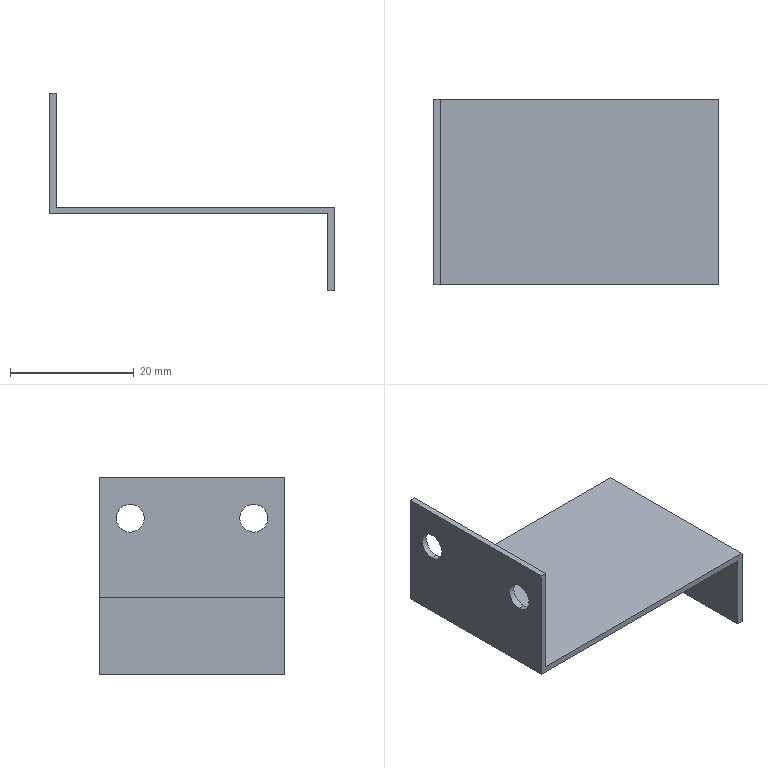Part | STEP file | 0244_221_Dog | 1 solid | 14 faces | box 46 x 30 x 32 mm | volume 2278 mm3 | plane 10 | cylinder 4 | commonest cylinder face diameters 4.5 x4
STEP:
#1=CARTESIAN_POINT('',(0.,0.,0.));
#2=DIRECTION('',(0.,0.,1.));
#3=DIRECTION('',(1.,0.,0.));
#4=AXIS2_PLACEMENT_3D('',#1,#2,#3);
#5=CARTESIAN_POINT('',(0.,10.,10.6));
#6=VERTEX_POINT('',#5);
#7=CARTESIAN_POINT('',(1.,10.,10.6));
#8=VERTEX_POINT('',#7);
#9=CARTESIAN_POINT('',(1.,10.,10.6));
#10=DIRECTION('',(1.,0.,0.));
#11=VECTOR('',#10,1.);
#12=LINE('',#9,#11);
#13=CARTESIAN_POINT('',(1.,10.,12.85));
#14=DIRECTION('',(1.,0.,0.));
#15=DIRECTION('',(0.,0.,-1.));
#16=AXIS2_PLACEMENT_3D('',#13,#14,#15);
#17=CYLINDRICAL_SURFACE('',#16,2.25);
#18=CARTESIAN_POINT('',(6.283,0.));
#19=DIRECTION('',(0.,1.));
#20=VECTOR('',#19,1.);
#21=LINE('',#18,#20);
#22=(GEOMETRIC_REPRESENTATION_CONTEXT(2)PARAMETRIC_REPRESENTATION_CONTEXT()REPRESENTATION_CONTEXT('',''));
#23=DEFINITIONAL_REPRESENTATION('',(#21),#22);
#24=PCURVE('',#17,#23);
#25=CARTESIAN_POINT('',(1.,10.,12.85));
#26=DIRECTION('',(1.,0.,0.));
#27=DIRECTION('',(0.,0.,-1.));
#28=AXIS2_PLACEMENT_3D('',#25,#26,#27);
#29=CYLINDRICAL_SURFACE('',#28,2.25);
#30=CARTESIAN_POINT('',(0.,0.));
#31=DIRECTION('',(0.,1.));
#32=VECTOR('',#31,1.);
#33=LINE('',#30,#32);
#34=(GEOMETRIC_REPRESENTATION_CONTEXT(2)PARAMETRIC_REPRESENTATION_CONTEXT()REPRESENTATION_CONTEXT('',''));
#35=DEFINITIONAL_REPRESENTATION('',(#33),#34);
#36=PCURVE('',#29,#35);
#37=SURFACE_CURVE('',#12,(#24,#36),.PCURVE_S1.);
#38=EDGE_CURVE('',#6,#8,#37,.T.);
#39=ORIENTED_EDGE('',*,*,#38,.T.);
#40=CARTESIAN_POINT('',(1.,10.,15.1));
#41=VERTEX_POINT('',#40);
#42=CARTESIAN_POINT('',(1.,10.,12.85));
#43=DIRECTION('',(1.,0.,0.));
#44=DIRECTION('',(0.,0.,-1.));
#45=AXIS2_PLACEMENT_3D('',#42,#43,#44);
#46=CIRCLE('',#45,2.25);
#47=CARTESIAN_POINT('',(0.,0.));
#48=DIRECTION('',(1.,0.));
#49=VECTOR('',#48,1.);
#50=LINE('',#47,#49);
#51=(GEOMETRIC_REPRESENTATION_CONTEXT(2)PARAMETRIC_REPRESENTATION_CONTEXT()REPRESENTATION_CONTEXT('',''));
#52=DEFINITIONAL_REPRESENTATION('',(#50),#51);
#53=PCURVE('',#17,#52);
#54=CARTESIAN_POINT('',(1.,15.,1.));
#55=DIRECTION('',(-1.,0.,0.));
#56=DIRECTION('',(0.,0.,1.));
#57=AXIS2_PLACEMENT_3D('',#54,#55,#56);
#58=PLANE('',#57);
#59=CARTESIAN_POINT('',(9.6,-5.));
#60=CARTESIAN_POINT('',(9.6,-1.103));
#61=CARTESIAN_POINT('',(12.975,-3.051));
#62=CARTESIAN_POINT('',(16.35,-5.));
#63=CARTESIAN_POINT('',(12.975,-6.949));
#64=CARTESIAN_POINT('',(9.6,-8.897));
#65=CARTESIAN_POINT('',(9.6,-5.));
#66=(BOUNDED_CURVE()B_SPLINE_CURVE(2,(#59,#60,#61,#62,#63,#64,#65),.UNSPECIFIED.,.T.,.F.)B_SPLINE_CURVE_WITH_KNOTS((1,2,2,2,2,1),(-2.094,0.,2.094,4.189,6.283,8.378),.UNSPECIFIED.)CURVE()GEOMETRIC_REPRESENTATION_ITEM()RATIONAL_B_SPLINE_CURVE((1.,0.5,1.,0.5,1.,0.5,1.))REPRESENTATION_ITEM(''));
#67=(GEOMETRIC_REPRESENTATION_CONTEXT(2)PARAMETRIC_REPRESENTATION_CONTEXT()REPRESENTATION_CONTEXT('',''));
#68=DEFINITIONAL_REPRESENTATION('',(#66),#67);
#69=PCURVE('',#58,#68);
#70=SURFACE_CURVE('',#46,(#53,#69),.PCURVE_S1.);
#71=EDGE_CURVE('',#41,#8,#70,.T.);
#72=ORIENTED_EDGE('',*,*,#71,.F.);
#73=CARTESIAN_POINT('',(0.,10.,15.1));
#74=VERTEX_POINT('',#73);
#75=CARTESIAN_POINT('',(1.,10.,15.1));
#76=DIRECTION('',(1.,0.,0.));
#77=VECTOR('',#76,1.);
#78=LINE('',#75,#77);
#79=CARTESIAN_POINT('',(3.142,0.));
#80=DIRECTION('',(0.,1.));
#81=VECTOR('',#80,1.);
#82=LINE('',#79,#81);
#83=(GEOMETRIC_REPRESENTATION_CONTEXT(2)PARAMETRIC_REPRESENTATION_CONTEXT()REPRESENTATION_CONTEXT('',''));
#84=DEFINITIONAL_REPRESENTATION('',(#82),#83);
#85=PCURVE('',#17,#84);
#86=CARTESIAN_POINT('',(3.142,0.));
#87=DIRECTION('',(0.,1.));
#88=VECTOR('',#87,1.);
#89=LINE('',#86,#88);
#90=(GEOMETRIC_REPRESENTATION_CONTEXT(2)PARAMETRIC_REPRESENTATION_CONTEXT()REPRESENTATION_CONTEXT('',''));
#91=DEFINITIONAL_REPRESENTATION('',(#89),#90);
#92=PCURVE('',#29,#91);
#93=SURFACE_CURVE('',#78,(#85,#92),.PCURVE_S1.);
#94=EDGE_CURVE('',#74,#41,#93,.T.);
#95=ORIENTED_EDGE('',*,*,#94,.F.);
#96=CARTESIAN_POINT('',(0.,10.,12.85));
#97=DIRECTION('',(1.,0.,0.));
#98=DIRECTION('',(0.,0.,-1.));
#99=AXIS2_PLACEMENT_3D('',#96,#97,#98);
#100=CIRCLE('',#99,2.25);
#101=CARTESIAN_POINT('',(0.,-1.));
#102=DIRECTION('',(1.,0.));
#103=VECTOR('',#102,1.);
#104=LINE('',#101,#103);
#105=(GEOMETRIC_REPRESENTATION_CONTEXT(2)PARAMETRIC_REPRESENTATION_CONTEXT()REPRESENTATION_CONTEXT('',''));
#106=DEFINITIONAL_REPRESENTATION('',(#104),#105);
#107=PCURVE('',#17,#106);
#108=CARTESIAN_POINT('',(0.,15.,0.));
#109=DIRECTION('',(1.,0.,0.));
#110=DIRECTION('',(0.,0.,-1.));
#111=AXIS2_PLACEMENT_3D('',#108,#109,#110);
#112=PLANE('',#111);
#113=CARTESIAN_POINT('',(-12.85,-5.));
#114=DIRECTION('',(1.,0.));
#115=AXIS2_PLACEMENT_2D('',#113,#114);
#116=CIRCLE('',#115,2.25);
#117=(GEOMETRIC_REPRESENTATION_CONTEXT(2)PARAMETRIC_REPRESENTATION_CONTEXT()REPRESENTATION_CONTEXT('',''));
#118=DEFINITIONAL_REPRESENTATION('',(#116),#117);
#119=PCURVE('',#112,#118);
#120=SURFACE_CURVE('',#100,(#107,#119),.PCURVE_S1.);
#121=EDGE_CURVE('',#74,#6,#120,.T.);
#122=ORIENTED_EDGE('',*,*,#121,.T.);
#123=EDGE_LOOP('',(#39,#72,#95,#122));
#124=FACE_BOUND('',#123,.F.);
#125=ADVANCED_FACE('',(#124),#17,.F.);
#126=CARTESIAN_POINT('',(0.,-10.,10.6));
#127=VERTEX_POINT('',#126);
#128=CARTESIAN_POINT('',(1.,-10.,10.6));
#129=VERTEX_POINT('',#128);
#130=CARTESIAN_POINT('',(1.,-10.,10.6));
#131=DIRECTION('',(1.,0.,0.));
#132=VECTOR('',#131,1.);
#133=LINE('',#130,#132);
#134=CARTESIAN_POINT('',(1.,-10.,12.85));
#135=DIRECTION('',(1.,0.,0.));
#136=DIRECTION('',(0.,0.,-1.));
#137=AXIS2_PLACEMENT_3D('',#134,#135,#136);
#138=CYLINDRICAL_SURFACE('',#137,2.25);
#139=CARTESIAN_POINT('',(6.283,0.));
#140=DIRECTION('',(0.,1.));
#141=VECTOR('',#140,1.);
#142=LINE('',#139,#141);
#143=(GEOMETRIC_REPRESENTATION_CONTEXT(2)PARAMETRIC_REPRESENTATION_CONTEXT()REPRESENTATION_CONTEXT('',''));
#144=DEFINITIONAL_REPRESENTATION('',(#142),#143);
#145=PCURVE('',#138,#144);
#146=CARTESIAN_POINT('',(1.,-10.,12.85));
#147=DIRECTION('',(1.,0.,0.));
#148=DIRECTION('',(0.,0.,-1.));
#149=AXIS2_PLACEMENT_3D('',#146,#147,#148);
#150=CYLINDRICAL_SURFACE('',#149,2.25);
#151=CARTESIAN_POINT('',(0.,0.));
#152=DIRECTION('',(0.,1.));
#153=VECTOR('',#152,1.);
#154=LINE('',#151,#153);
#155=(GEOMETRIC_REPRESENTATION_CONTEXT(2)PARAMETRIC_REPRESENTATION_CONTEXT()REPRESENTATION_CONTEXT('',''));
#156=DEFINITIONAL_REPRESENTATION('',(#154),#155);
#157=PCURVE('',#150,#156);
#158=SURFACE_CURVE('',#133,(#145,#157),.PCURVE_S1.);
#159=EDGE_CURVE('',#127,#129,#158,.T.);
#160=ORIENTED_EDGE('',*,*,#159,.T.);
#161=CARTESIAN_POINT('',(1.,-10.,15.1));
#162=VERTEX_POINT('',#161);
#163=CARTESIAN_POINT('',(1.,-10.,12.85));
#164=DIRECTION('',(1.,0.,0.));
#165=DIRECTION('',(0.,0.,-1.));
#166=AXIS2_PLACEMENT_3D('',#163,#164,#165);
#167=CIRCLE('',#166,2.25);
#168=CARTESIAN_POINT('',(0.,0.));
#169=DIRECTION('',(1.,0.));
#170=VECTOR('',#169,1.);
#171=LINE('',#168,#170);
#172=(GEOMETRIC_REPRESENTATION_CONTEXT(2)PARAMETRIC_REPRESENTATION_CONTEXT()REPRESENTATION_CONTEXT('',''));
#173=DEFINITIONAL_REPRESENTATION('',(#171),#172);
#174=PCURVE('',#138,#173);
#175=CARTESIAN_POINT('',(9.6,-25.));
#176=CARTESIAN_POINT('',(9.6,-21.103));
#177=CARTESIAN_POINT('',(12.975,-23.051));
#178=CARTESIAN_POINT('',(16.35,-25.));
#179=CARTESIAN_POINT('',(12.975,-26.949));
#180=CARTESIAN_POINT('',(9.6,-28.897));
#181=CARTESIAN_POINT('',(9.6,-25.));
#182=(BOUNDED_CURVE()B_SPLINE_CURVE(2,(#175,#176,#177,#178,#179,#180,#181),.UNSPECIFIED.,.T.,.F.)B_SPLINE_CURVE_WITH_KNOTS((1,2,2,2,2,1),(-2.094,0.,2.094,4.189,6.283,8.378),.UNSPECIFIED.)CURVE()GEOMETRIC_REPRESENTATION_ITEM()RATIONAL_B_SPLINE_CURVE((1.,0.5,1.,0.5,1.,0.5,1.))REPRESENTATION_ITEM(''));
#183=(GEOMETRIC_REPRESENTATION_CONTEXT(2)PARAMETRIC_REPRESENTATION_CONTEXT()REPRESENTATION_CONTEXT('',''));
#184=DEFINITIONAL_REPRESENTATION('',(#182),#183);
#185=PCURVE('',#58,#184);
#186=SURFACE_CURVE('',#167,(#174,#185),.PCURVE_S1.);
#187=EDGE_CURVE('',#162,#129,#186,.T.);
#188=ORIENTED_EDGE('',*,*,#187,.F.);
#189=CARTESIAN_POINT('',(0.,-10.,15.1));
#190=VERTEX_POINT('',#189);
#191=CARTESIAN_POINT('',(1.,-10.,15.1));
#192=DIRECTION('',(1.,0.,0.));
#193=VECTOR('',#192,1.);
#194=LINE('',#191,#193);
#195=CARTESIAN_POINT('',(3.142,0.));
#196=DIRECTION('',(0.,1.));
#197=VECTOR('',#196,1.);
#198=LINE('',#195,#197);
#199=(GEOMETRIC_REPRESENTATION_CONTEXT(2)PARAMETRIC_REPRESENTATION_CONTEXT()REPRESENTATION_CONTEXT('',''));
#200=DEFINITIONAL_REPRESENTATION('',(#198),#199);
#201=PCURVE('',#138,#200);
#202=CARTESIAN_POINT('',(3.142,0.));
#203=DIRECTION('',(0.,1.));
#204=VECTOR('',#203,1.);
#205=LINE('',#202,#204);
#206=(GEOMETRIC_REPRESENTATION_CONTEXT(2)PARAMETRIC_REPRESENTATION_CONTEXT()REPRESENTATION_CONTEXT('',''));
#207=DEFINITIONAL_REPRESENTATION('',(#205),#206);
#208=PCURVE('',#150,#207);
#209=SURFACE_CURVE('',#194,(#201,#208),.PCURVE_S1.);
#210=EDGE_CURVE('',#190,#162,#209,.T.);
#211=ORIENTED_EDGE('',*,*,#210,.F.);
#212=CARTESIAN_POINT('',(0.,-10.,12.85));
#213=DIRECTION('',(1.,0.,0.));
#214=DIRECTION('',(0.,0.,-1.));
#215=AXIS2_PLACEMENT_3D('',#212,#213,#214);
#216=CIRCLE('',#215,2.25);
#217=CARTESIAN_POINT('',(0.,-1.));
#218=DIRECTION('',(1.,0.));
#219=VECTOR('',#218,1.);
#220=LINE('',#217,#219);
#221=(GEOMETRIC_REPRESENTATION_CONTEXT(2)PARAMETRIC_REPRESENTATION_CONTEXT()REPRESENTATION_CONTEXT('',''));
#222=DEFINITIONAL_REPRESENTATION('',(#220),#221);
#223=PCURVE('',#138,#222);
#224=CARTESIAN_POINT('',(-12.85,-25.));
#225=DIRECTION('',(1.,0.));
#226=AXIS2_PLACEMENT_2D('',#224,#225);
#227=CIRCLE('',#226,2.25);
#228=(GEOMETRIC_REPRESENTATION_CONTEXT(2)PARAMETRIC_REPRESENTATION_CONTEXT()REPRESENTATION_CONTEXT('',''));
#229=DEFINITIONAL_REPRESENTATION('',(#227),#228);
#230=PCURVE('',#112,#229);
#231=SURFACE_CURVE('',#216,(#223,#230),.PCURVE_S1.);
#232=EDGE_CURVE('',#190,#127,#231,.T.);
#233=ORIENTED_EDGE('',*,*,#232,.T.);
#234=EDGE_LOOP('',(#160,#188,#211,#233));
#235=FACE_BOUND('',#234,.F.);
#236=ADVANCED_FACE('',(#235),#138,.F.);
#237=CARTESIAN_POINT('',(1.,-15.,19.5));
#238=VERTEX_POINT('',#237);
#239=CARTESIAN_POINT('',(1.,-15.,1.));
#240=VERTEX_POINT('',#239);
#241=CARTESIAN_POINT('',(1.,-15.,1.));
#242=DIRECTION('',(0.,0.,-1.));
#243=VECTOR('',#242,1.);
#244=LINE('',#241,#243);
#245=CARTESIAN_POINT('',(0.,-30.));
#246=DIRECTION('',(-1.,0.));
#247=VECTOR('',#246,1.);
#248=LINE('',#245,#247);
#249=(GEOMETRIC_REPRESENTATION_CONTEXT(2)PARAMETRIC_REPRESENTATION_CONTEXT()REPRESENTATION_CONTEXT('',''));
#250=DEFINITIONAL_REPRESENTATION('',(#248),#249);
#251=PCURVE('',#58,#250);
#252=CARTESIAN_POINT('',(45.,-15.,0.));
#253=DIRECTION('',(0.,1.,0.));
#254=DIRECTION('',(0.,0.,1.));
#255=AXIS2_PLACEMENT_3D('',#252,#253,#254);
#256=PLANE('',#255);
#257=CARTESIAN_POINT('',(1.,-44.));
#258=DIRECTION('',(-1.,0.));
#259=VECTOR('',#258,1.);
#260=LINE('',#257,#259);
#261=(GEOMETRIC_REPRESENTATION_CONTEXT(2)PARAMETRIC_REPRESENTATION_CONTEXT()REPRESENTATION_CONTEXT('',''));
#262=DEFINITIONAL_REPRESENTATION('',(#260),#261);
#263=PCURVE('',#256,#262);
#264=SURFACE_CURVE('',#244,(#251,#263),.PCURVE_S1.);
#265=EDGE_CURVE('',#238,#240,#264,.T.);
#266=ORIENTED_EDGE('',*,*,#265,.T.);
#267=CARTESIAN_POINT('',(1.,15.,1.));
#268=VERTEX_POINT('',#267);
#269=CARTESIAN_POINT('',(1.,15.,1.));
#270=DIRECTION('',(0.,-1.,0.));
#271=VECTOR('',#270,1.);
#272=LINE('',#269,#271);
#273=CARTESIAN_POINT('',(0.,0.));
#274=DIRECTION('',(0.,-1.));
#275=VECTOR('',#274,1.);
#276=LINE('',#273,#275);
#277=(GEOMETRIC_REPRESENTATION_CONTEXT(2)PARAMETRIC_REPRESENTATION_CONTEXT()REPRESENTATION_CONTEXT('',''));
#278=DEFINITIONAL_REPRESENTATION('',(#276),#277);
#279=PCURVE('',#58,#278);
#280=CARTESIAN_POINT('',(1.,15.,1.));
#281=DIRECTION('',(0.,0.,-1.));
#282=DIRECTION('',(-1.,0.,0.));
#283=AXIS2_PLACEMENT_3D('',#280,#281,#282);
#284=PLANE('',#283);
#285=CARTESIAN_POINT('',(0.,0.));
#286=DIRECTION('',(0.,-1.));
#287=VECTOR('',#286,1.);
#288=LINE('',#285,#287);
#289=(GEOMETRIC_REPRESENTATION_CONTEXT(2)PARAMETRIC_REPRESENTATION_CONTEXT()REPRESENTATION_CONTEXT('',''));
#290=DEFINITIONAL_REPRESENTATION('',(#288),#289);
#291=PCURVE('',#284,#290);
#292=SURFACE_CURVE('',#272,(#279,#291),.PCURVE_S1.);
#293=EDGE_CURVE('',#268,#240,#292,.T.);
#294=ORIENTED_EDGE('',*,*,#293,.F.);
#295=CARTESIAN_POINT('',(1.,15.,19.5));
#296=VERTEX_POINT('',#295);
#297=CARTESIAN_POINT('',(1.,15.,1.));
#298=DIRECTION('',(0.,0.,-1.));
#299=VECTOR('',#298,1.);
#300=LINE('',#297,#299);
#301=CARTESIAN_POINT('',(0.,0.));
#302=DIRECTION('',(-1.,0.));
#303=VECTOR('',#302,1.);
#304=LINE('',#301,#303);
#305=(GEOMETRIC_REPRESENTATION_CONTEXT(2)PARAMETRIC_REPRESENTATION_CONTEXT()REPRESENTATION_CONTEXT('',''));
#306=DEFINITIONAL_REPRESENTATION('',(#304),#305);
#307=PCURVE('',#58,#306);
#308=CARTESIAN_POINT('',(45.,15.,0.));
#309=DIRECTION('',(0.,1.,0.));
#310=DIRECTION('',(0.,0.,1.));
#311=AXIS2_PLACEMENT_3D('',#308,#309,#310);
#312=PLANE('',#311);
#313=CARTESIAN_POINT('',(1.,-44.));
#314=DIRECTION('',(-1.,0.));
#315=VECTOR('',#314,1.);
#316=LINE('',#313,#315);
#317=(GEOMETRIC_REPRESENTATION_CONTEXT(2)PARAMETRIC_REPRESENTATION_CONTEXT()REPRESENTATION_CONTEXT('',''));
#318=DEFINITIONAL_REPRESENTATION('',(#316),#317);
#319=PCURVE('',#312,#318);
#320=SURFACE_CURVE('',#300,(#307,#319),.PCURVE_S1.);
#321=EDGE_CURVE('',#296,#268,#320,.T.);
#322=ORIENTED_EDGE('',*,*,#321,.F.);
#323=CARTESIAN_POINT('',(1.,15.,19.5));
#324=DIRECTION('',(0.,-1.,0.));
#325=VECTOR('',#324,1.);
#326=LINE('',#323,#325);
#327=CARTESIAN_POINT('',(18.5,0.));
#328=DIRECTION('',(0.,-1.));
#329=VECTOR('',#328,1.);
#330=LINE('',#327,#329);
#331=(GEOMETRIC_REPRESENTATION_CONTEXT(2)PARAMETRIC_REPRESENTATION_CONTEXT()REPRESENTATION_CONTEXT('',''));
#332=DEFINITIONAL_REPRESENTATION('',(#330),#331);
#333=PCURVE('',#58,#332);
#334=CARTESIAN_POINT('',(0.,15.,19.5));
#335=DIRECTION('',(0.,0.,-1.));
#336=DIRECTION('',(-1.,0.,0.));
#337=AXIS2_PLACEMENT_3D('',#334,#335,#336);
#338=PLANE('',#337);
#339=CARTESIAN_POINT('',(-1.,0.));
#340=DIRECTION('',(0.,-1.));
#341=VECTOR('',#340,1.);
#342=LINE('',#339,#341);
#343=(GEOMETRIC_REPRESENTATION_CONTEXT(2)PARAMETRIC_REPRESENTATION_CONTEXT()REPRESENTATION_CONTEXT('',''));
#344=DEFINITIONAL_REPRESENTATION('',(#342),#343);
#345=PCURVE('',#338,#344);
#346=SURFACE_CURVE('',#326,(#333,#345),.PCURVE_S1.);
#347=EDGE_CURVE('',#296,#238,#346,.T.);
#348=ORIENTED_EDGE('',*,*,#347,.T.);
#349=EDGE_LOOP('',(#266,#294,#322,#348));
#350=FACE_BOUND('',#349,.T.);
#351=CARTESIAN_POINT('',(1.,-10.,12.85));
#352=DIRECTION('',(1.,0.,0.));
#353=DIRECTION('',(0.,0.,-1.));
#354=AXIS2_PLACEMENT_3D('',#351,#352,#353);
#355=CIRCLE('',#354,2.25);
#356=CARTESIAN_POINT('',(9.6,-25.));
#357=CARTESIAN_POINT('',(9.6,-21.103));
#358=CARTESIAN_POINT('',(12.975,-23.051));
#359=CARTESIAN_POINT('',(16.35,-25.));
#360=CARTESIAN_POINT('',(12.975,-26.949));
#361=CARTESIAN_POINT('',(9.6,-28.897));
#362=CARTESIAN_POINT('',(9.6,-25.));
#363=(BOUNDED_CURVE()B_SPLINE_CURVE(2,(#356,#357,#358,#359,#360,#361,#362),.UNSPECIFIED.,.T.,.F.)B_SPLINE_CURVE_WITH_KNOTS((1,2,2,2,2,1),(-2.094,0.,2.094,4.189,6.283,8.378),.UNSPECIFIED.)CURVE()GEOMETRIC_REPRESENTATION_ITEM()RATIONAL_B_SPLINE_CURVE((1.,0.5,1.,0.5,1.,0.5,1.))REPRESENTATION_ITEM(''));
#364=(GEOMETRIC_REPRESENTATION_CONTEXT(2)PARAMETRIC_REPRESENTATION_CONTEXT()REPRESENTATION_CONTEXT('',''));
#365=DEFINITIONAL_REPRESENTATION('',(#363),#364);
#366=PCURVE('',#58,#365);
#367=CARTESIAN_POINT('',(0.,0.));
#368=DIRECTION('',(1.,0.));
#369=VECTOR('',#368,1.);
#370=LINE('',#367,#369);
#371=(GEOMETRIC_REPRESENTATION_CONTEXT(2)PARAMETRIC_REPRESENTATION_CONTEXT()REPRESENTATION_CONTEXT('',''));
#372=DEFINITIONAL_REPRESENTATION('',(#370),#371);
#373=PCURVE('',#150,#372);
#374=SURFACE_CURVE('',#355,(#366,#373),.PCURVE_S1.);
#375=EDGE_CURVE('',#129,#162,#374,.T.);
#376=ORIENTED_EDGE('',*,*,#375,.F.);
#377=ORIENTED_EDGE('',*,*,#187,.F.);
#378=EDGE_LOOP('',(#376,#377));
#379=FACE_BOUND('',#378,.T.);
#380=CARTESIAN_POINT('',(1.,10.,12.85));
#381=DIRECTION('',(1.,0.,0.));
#382=DIRECTION('',(0.,0.,-1.));
#383=AXIS2_PLACEMENT_3D('',#380,#381,#382);
#384=CIRCLE('',#383,2.25);
#385=CARTESIAN_POINT('',(9.6,-5.));
#386=CARTESIAN_POINT('',(9.6,-1.103));
#387=CARTESIAN_POINT('',(12.975,-3.051));
#388=CARTESIAN_POINT('',(16.35,-5.));
#389=CARTESIAN_POINT('',(12.975,-6.949));
#390=CARTESIAN_POINT('',(9.6,-8.897));
#391=CARTESIAN_POINT('',(9.6,-5.));
#392=(BOUNDED_CURVE()B_SPLINE_CURVE(2,(#385,#386,#387,#388,#389,#390,#391),.UNSPECIFIED.,.T.,.F.)B_SPLINE_CURVE_WITH_KNOTS((1,2,2,2,2,1),(-2.094,0.,2.094,4.189,6.283,8.378),.UNSPECIFIED.)CURVE()GEOMETRIC_REPRESENTATION_ITEM()RATIONAL_B_SPLINE_CURVE((1.,0.5,1.,0.5,1.,0.5,1.))REPRESENTATION_ITEM(''));
#393=(GEOMETRIC_REPRESENTATION_CONTEXT(2)PARAMETRIC_REPRESENTATION_CONTEXT()REPRESENTATION_CONTEXT('',''));
#394=DEFINITIONAL_REPRESENTATION('',(#392),#393);
#395=PCURVE('',#58,#394);
#396=CARTESIAN_POINT('',(0.,0.));
#397=DIRECTION('',(1.,0.));
#398=VECTOR('',#397,1.);
#399=LINE('',#396,#398);
#400=(GEOMETRIC_REPRESENTATION_CONTEXT(2)PARAMETRIC_REPRESENTATION_CONTEXT()REPRESENTATION_CONTEXT('',''));
#401=DEFINITIONAL_REPRESENTATION('',(#399),#400);
#402=PCURVE('',#29,#401);
#403=SURFACE_CURVE('',#384,(#395,#402),.PCURVE_S1.);
#404=EDGE_CURVE('',#8,#41,#403,.T.);
#405=ORIENTED_EDGE('',*,*,#404,.F.);
#406=ORIENTED_EDGE('',*,*,#71,.F.);
#407=EDGE_LOOP('',(#405,#406));
#408=FACE_BOUND('',#407,.T.);
#409=ADVANCED_FACE('',(#350,#379,#408),#58,.F.);
#410=CARTESIAN_POINT('',(45.,-15.,0.));
#411=VERTEX_POINT('',#410);
#412=CARTESIAN_POINT('',(0.,-15.,0.));
#413=VERTEX_POINT('',#412);
#414=CARTESIAN_POINT('',(0.,-15.,0.));
#415=DIRECTION('',(-1.,0.,0.));
#416=VECTOR('',#415,1.);
#417=LINE('',#414,#416);
#418=CARTESIAN_POINT('',(0.,15.,0.));
#419=DIRECTION('',(0.,0.,1.));
#420=DIRECTION('',(1.,0.,0.));
#421=AXIS2_PLACEMENT_3D('',#418,#419,#420);
#422=PLANE('',#421);
#423=CARTESIAN_POINT('',(0.,-30.));
#424=DIRECTION('',(-1.,0.));
#425=VECTOR('',#424,1.);
#426=LINE('',#423,#425);
#427=(GEOMETRIC_REPRESENTATION_CONTEXT(2)PARAMETRIC_REPRESENTATION_CONTEXT()REPRESENTATION_CONTEXT('',''));
#428=DEFINITIONAL_REPRESENTATION('',(#426),#427);
#429=PCURVE('',#422,#428);
#430=CARTESIAN_POINT('',(0.,-45.));
#431=DIRECTION('',(0.,-1.));
#432=VECTOR('',#431,1.);
#433=LINE('',#430,#432);
#434=(GEOMETRIC_REPRESENTATION_CONTEXT(2)PARAMETRIC_REPRESENTATION_CONTEXT()REPRESENTATION_CONTEXT('',''));
#435=DEFINITIONAL_REPRESENTATION('',(#433),#434);
#436=PCURVE('',#256,#435);
#437=SURFACE_CURVE('',#417,(#429,#436),.PCURVE_S1.);
#438=EDGE_CURVE('',#411,#413,#437,.T.);
#439=ORIENTED_EDGE('',*,*,#438,.T.);
#440=CARTESIAN_POINT('',(0.,15.,0.));
#441=VERTEX_POINT('',#440);
#442=CARTESIAN_POINT('',(0.,15.,0.));
#443=DIRECTION('',(0.,-1.,0.));
#444=VECTOR('',#443,1.);
#445=LINE('',#442,#444);
#446=CARTESIAN_POINT('',(0.,0.));
#447=DIRECTION('',(0.,-1.));
#448=VECTOR('',#447,1.);
#449=LINE('',#446,#448);
#450=(GEOMETRIC_REPRESENTATION_CONTEXT(2)PARAMETRIC_REPRESENTATION_CONTEXT()REPRESENTATION_CONTEXT('',''));
#451=DEFINITIONAL_REPRESENTATION('',(#449),#450);
#452=PCURVE('',#422,#451);
#453=CARTESIAN_POINT('',(0.,0.));
#454=DIRECTION('',(0.,-1.));
#455=VECTOR('',#454,1.);
#456=LINE('',#453,#455);
#457=(GEOMETRIC_REPRESENTATION_CONTEXT(2)PARAMETRIC_REPRESENTATION_CONTEXT()REPRESENTATION_CONTEXT('',''));
#458=DEFINITIONAL_REPRESENTATION('',(#456),#457);
#459=PCURVE('',#112,#458);
#460=SURFACE_CURVE('',#445,(#452,#459),.PCURVE_S1.);
#461=EDGE_CURVE('',#441,#413,#460,.T.);
#462=ORIENTED_EDGE('',*,*,#461,.F.);
#463=CARTESIAN_POINT('',(45.,15.,0.));
#464=VERTEX_POINT('',#463);
#465=CARTESIAN_POINT('',(0.,15.,0.));
#466=DIRECTION('',(-1.,0.,0.));
#467=VECTOR('',#466,1.);
#468=LINE('',#465,#467);
#469=CARTESIAN_POINT('',(0.,0.));
#470=DIRECTION('',(-1.,0.));
#471=VECTOR('',#470,1.);
#472=LINE('',#469,#471);
#473=(GEOMETRIC_REPRESENTATION_CONTEXT(2)PARAMETRIC_REPRESENTATION_CONTEXT()REPRESENTATION_CONTEXT('',''));
#474=DEFINITIONAL_REPRESENTATION('',(#472),#473);
#475=PCURVE('',#422,#474);
#476=CARTESIAN_POINT('',(0.,-45.));
#477=DIRECTION('',(0.,-1.));
#478=VECTOR('',#477,1.);
#479=LINE('',#476,#478);
#480=(GEOMETRIC_REPRESENTATION_CONTEXT(2)PARAMETRIC_REPRESENTATION_CONTEXT()REPRESENTATION_CONTEXT('',''));
#481=DEFINITIONAL_REPRESENTATION('',(#479),#480);
#482=PCURVE('',#312,#481);
#483=SURFACE_CURVE('',#468,(#475,#482),.PCURVE_S1.);
#484=EDGE_CURVE('',#464,#441,#483,.T.);
#485=ORIENTED_EDGE('',*,*,#484,.F.);
#486=CARTESIAN_POINT('',(45.,15.,0.));
#487=DIRECTION('',(0.,-1.,0.));
#488=VECTOR('',#487,1.);
#489=LINE('',#486,#488);
#490=CARTESIAN_POINT('',(45.,0.));
#491=DIRECTION('',(0.,-1.));
#492=VECTOR('',#491,1.);
#493=LINE('',#490,#492);
#494=(GEOMETRIC_REPRESENTATION_CONTEXT(2)PARAMETRIC_REPRESENTATION_CONTEXT()REPRESENTATION_CONTEXT('',''));
#495=DEFINITIONAL_REPRESENTATION('',(#493),#494);
#496=PCURVE('',#422,#495);
#497=CARTESIAN_POINT('',(45.,15.,0.));
#498=DIRECTION('',(1.,0.,0.));
#499=DIRECTION('',(0.,0.,-1.));
#500=AXIS2_PLACEMENT_3D('',#497,#498,#499);
#501=PLANE('',#500);
#502=CARTESIAN_POINT('',(0.,0.));
#503=DIRECTION('',(0.,-1.));
#504=VECTOR('',#503,1.);
#505=LINE('',#502,#504);
#506=(GEOMETRIC_REPRESENTATION_CONTEXT(2)PARAMETRIC_REPRESENTATION_CONTEXT()REPRESENTATION_CONTEXT('',''));
#507=DEFINITIONAL_REPRESENTATION('',(#505),#506);
#508=PCURVE('',#501,#507);
#509=SURFACE_CURVE('',#489,(#496,#508),.PCURVE_S1.);
#510=EDGE_CURVE('',#464,#411,#509,.T.);
#511=ORIENTED_EDGE('',*,*,#510,.T.);
#512=EDGE_LOOP('',(#439,#462,#485,#511));
#513=FACE_BOUND('',#512,.T.);
#514=ADVANCED_FACE('',(#513),#422,.F.);
#515=CARTESIAN_POINT('',(0.,10.,12.85));
#516=DIRECTION('',(1.,0.,0.));
#517=DIRECTION('',(0.,0.,-1.));
#518=AXIS2_PLACEMENT_3D('',#515,#516,#517);
#519=CIRCLE('',#518,2.25);
#520=CARTESIAN_POINT('',(-12.85,-5.));
#521=DIRECTION('',(1.,0.));
#522=AXIS2_PLACEMENT_2D('',#520,#521);
#523=CIRCLE('',#522,2.25);
#524=(GEOMETRIC_REPRESENTATION_CONTEXT(2)PARAMETRIC_REPRESENTATION_CONTEXT()REPRESENTATION_CONTEXT('',''));
#525=DEFINITIONAL_REPRESENTATION('',(#523),#524);
#526=PCURVE('',#112,#525);
#527=CARTESIAN_POINT('',(0.,-1.));
#528=DIRECTION('',(1.,0.));
#529=VECTOR('',#528,1.);
#530=LINE('',#527,#529);
#531=(GEOMETRIC_REPRESENTATION_CONTEXT(2)PARAMETRIC_REPRESENTATION_CONTEXT()REPRESENTATION_CONTEXT('',''));
#532=DEFINITIONAL_REPRESENTATION('',(#530),#531);
#533=PCURVE('',#29,#532);
#534=SURFACE_CURVE('',#519,(#526,#533),.PCURVE_S1.);
#535=EDGE_CURVE('',#6,#74,#534,.T.);
#536=ORIENTED_EDGE('',*,*,#535,.T.);
#537=ORIENTED_EDGE('',*,*,#121,.T.);
#538=EDGE_LOOP('',(#536,#537));
#539=FACE_BOUND('',#538,.T.);
#540=CARTESIAN_POINT('',(0.,-10.,12.85));
#541=DIRECTION('',(1.,0.,0.));
#542=DIRECTION('',(0.,0.,-1.));
#543=AXIS2_PLACEMENT_3D('',#540,#541,#542);
#544=CIRCLE('',#543,2.25);
#545=CARTESIAN_POINT('',(-12.85,-25.));
#546=DIRECTION('',(1.,0.));
#547=AXIS2_PLACEMENT_2D('',#545,#546);
#548=CIRCLE('',#547,2.25);
#549=(GEOMETRIC_REPRESENTATION_CONTEXT(2)PARAMETRIC_REPRESENTATION_CONTEXT()REPRESENTATION_CONTEXT('',''));
#550=DEFINITIONAL_REPRESENTATION('',(#548),#549);
#551=PCURVE('',#112,#550);
#552=CARTESIAN_POINT('',(0.,-1.));
#553=DIRECTION('',(1.,0.));
#554=VECTOR('',#553,1.);
#555=LINE('',#552,#554);
#556=(GEOMETRIC_REPRESENTATION_CONTEXT(2)PARAMETRIC_REPRESENTATION_CONTEXT()REPRESENTATION_CONTEXT('',''));
#557=DEFINITIONAL_REPRESENTATION('',(#555),#556);
#558=PCURVE('',#150,#557);
#559=SURFACE_CURVE('',#544,(#551,#558),.PCURVE_S1.);
#560=EDGE_CURVE('',#127,#190,#559,.T.);
#561=ORIENTED_EDGE('',*,*,#560,.T.);
#562=ORIENTED_EDGE('',*,*,#232,.T.);
#563=EDGE_LOOP('',(#561,#562));
#564=FACE_BOUND('',#563,.T.);
#565=CARTESIAN_POINT('',(0.,-15.,19.5));
#566=VERTEX_POINT('',#565);
#567=CARTESIAN_POINT('',(0.,-15.,0.));
#568=DIRECTION('',(0.,0.,1.));
#569=VECTOR('',#568,1.);
#570=LINE('',#567,#569);
#571=CARTESIAN_POINT('',(0.,-30.));
#572=DIRECTION('',(-1.,0.));
#573=VECTOR('',#572,1.);
#574=LINE('',#571,#573);
#575=(GEOMETRIC_REPRESENTATION_CONTEXT(2)PARAMETRIC_REPRESENTATION_CONTEXT()REPRESENTATION_CONTEXT('',''));
#576=DEFINITIONAL_REPRESENTATION('',(#574),#575);
#577=PCURVE('',#112,#576);
#578=CARTESIAN_POINT('',(0.,-45.));
#579=DIRECTION('',(1.,0.));
#580=VECTOR('',#579,1.);
#581=LINE('',#578,#580);
#582=(GEOMETRIC_REPRESENTATION_CONTEXT(2)PARAMETRIC_REPRESENTATION_CONTEXT()REPRESENTATION_CONTEXT('',''));
#583=DEFINITIONAL_REPRESENTATION('',(#581),#582);
#584=PCURVE('',#256,#583);
#585=SURFACE_CURVE('',#570,(#577,#584),.PCURVE_S1.);
#586=EDGE_CURVE('',#413,#566,#585,.T.);
#587=ORIENTED_EDGE('',*,*,#586,.T.);
#588=CARTESIAN_POINT('',(0.,15.,19.5));
#589=VERTEX_POINT('',#588);
#590=CARTESIAN_POINT('',(0.,15.,19.5));
#591=DIRECTION('',(0.,-1.,0.));
#592=VECTOR('',#591,1.);
#593=LINE('',#590,#592);
#594=CARTESIAN_POINT('',(-19.5,0.));
#595=DIRECTION('',(0.,-1.));
#596=VECTOR('',#595,1.);
#597=LINE('',#594,#596);
#598=(GEOMETRIC_REPRESENTATION_CONTEXT(2)PARAMETRIC_REPRESENTATION_CONTEXT()REPRESENTATION_CONTEXT('',''));
#599=DEFINITIONAL_REPRESENTATION('',(#597),#598);
#600=PCURVE('',#112,#599);
#601=CARTESIAN_POINT('',(0.,0.));
#602=DIRECTION('',(0.,-1.));
#603=VECTOR('',#602,1.);
#604=LINE('',#601,#603);
#605=(GEOMETRIC_REPRESENTATION_CONTEXT(2)PARAMETRIC_REPRESENTATION_CONTEXT()REPRESENTATION_CONTEXT('',''));
#606=DEFINITIONAL_REPRESENTATION('',(#604),#605);
#607=PCURVE('',#338,#606);
#608=SURFACE_CURVE('',#593,(#600,#607),.PCURVE_S1.);
#609=EDGE_CURVE('',#589,#566,#608,.T.);
#610=ORIENTED_EDGE('',*,*,#609,.F.);
#611=CARTESIAN_POINT('',(0.,15.,0.));
#612=DIRECTION('',(0.,0.,1.));
#613=VECTOR('',#612,1.);
#614=LINE('',#611,#613);
#615=CARTESIAN_POINT('',(0.,0.));
#616=DIRECTION('',(-1.,0.));
#617=VECTOR('',#616,1.);
#618=LINE('',#615,#617);
#619=(GEOMETRIC_REPRESENTATION_CONTEXT(2)PARAMETRIC_REPRESENTATION_CONTEXT()REPRESENTATION_CONTEXT('',''));
#620=DEFINITIONAL_REPRESENTATION('',(#618),#619);
#621=PCURVE('',#112,#620);
#622=CARTESIAN_POINT('',(0.,-45.));
#623=DIRECTION('',(1.,0.));
#624=VECTOR('',#623,1.);
#625=LINE('',#622,#624);
#626=(GEOMETRIC_REPRESENTATION_CONTEXT(2)PARAMETRIC_REPRESENTATION_CONTEXT()REPRESENTATION_CONTEXT('',''));
#627=DEFINITIONAL_REPRESENTATION('',(#625),#626);
#628=PCURVE('',#312,#627);
#629=SURFACE_CURVE('',#614,(#621,#628),.PCURVE_S1.);
#630=EDGE_CURVE('',#441,#589,#629,.T.);
#631=ORIENTED_EDGE('',*,*,#630,.F.);
#632=ORIENTED_EDGE('',*,*,#461,.T.);
#633=EDGE_LOOP('',(#587,#610,#631,#632));
#634=FACE_BOUND('',#633,.T.);
#635=ADVANCED_FACE('',(#539,#564,#634),#112,.F.);
#636=CARTESIAN_POINT('',(0.,-15.,19.5));
#637=DIRECTION('',(1.,0.,0.));
#638=VECTOR('',#637,1.);
#639=LINE('',#636,#638);
#640=CARTESIAN_POINT('',(0.,-30.));
#641=DIRECTION('',(-1.,0.));
#642=VECTOR('',#641,1.);
#643=LINE('',#640,#642);
#644=(GEOMETRIC_REPRESENTATION_CONTEXT(2)PARAMETRIC_REPRESENTATION_CONTEXT()REPRESENTATION_CONTEXT('',''));
#645=DEFINITIONAL_REPRESENTATION('',(#643),#644);
#646=PCURVE('',#338,#645);
#647=CARTESIAN_POINT('',(19.5,-45.));
#648=DIRECTION('',(0.,1.));
#649=VECTOR('',#648,1.);
#650=LINE('',#647,#649);
#651=(GEOMETRIC_REPRESENTATION_CONTEXT(2)PARAMETRIC_REPRESENTATION_CONTEXT()REPRESENTATION_CONTEXT('',''));
#652=DEFINITIONAL_REPRESENTATION('',(#650),#651);
#653=PCURVE('',#256,#652);
#654=SURFACE_CURVE('',#639,(#646,#653),.PCURVE_S1.);
#655=EDGE_CURVE('',#566,#238,#654,.T.);
#656=ORIENTED_EDGE('',*,*,#655,.T.);
#657=ORIENTED_EDGE('',*,*,#347,.F.);
#658=CARTESIAN_POINT('',(0.,15.,19.5));
#659=DIRECTION('',(1.,0.,0.));
#660=VECTOR('',#659,1.);
#661=LINE('',#658,#660);
#662=CARTESIAN_POINT('',(0.,0.));
#663=DIRECTION('',(-1.,0.));
#664=VECTOR('',#663,1.);
#665=LINE('',#662,#664);
#666=(GEOMETRIC_REPRESENTATION_CONTEXT(2)PARAMETRIC_REPRESENTATION_CONTEXT()REPRESENTATION_CONTEXT('',''));
#667=DEFINITIONAL_REPRESENTATION('',(#665),#666);
#668=PCURVE('',#338,#667);
#669=CARTESIAN_POINT('',(19.5,-45.));
#670=DIRECTION('',(0.,1.));
#671=VECTOR('',#670,1.);
#672=LINE('',#669,#671);
#673=(GEOMETRIC_REPRESENTATION_CONTEXT(2)PARAMETRIC_REPRESENTATION_CONTEXT()REPRESENTATION_CONTEXT('',''));
#674=DEFINITIONAL_REPRESENTATION('',(#672),#673);
#675=PCURVE('',#312,#674);
#676=SURFACE_CURVE('',#661,(#668,#675),.PCURVE_S1.);
#677=EDGE_CURVE('',#589,#296,#676,.T.);
#678=ORIENTED_EDGE('',*,*,#677,.F.);
#679=ORIENTED_EDGE('',*,*,#609,.T.);
#680=EDGE_LOOP('',(#656,#657,#678,#679));
#681=FACE_BOUND('',#680,.T.);
#682=ADVANCED_FACE('',(#681),#338,.F.);
#683=CARTESIAN_POINT('',(46.,-15.,1.));
#684=VERTEX_POINT('',#683);
#685=CARTESIAN_POINT('',(1.,-15.,1.));
#686=DIRECTION('',(1.,0.,0.));
#687=VECTOR('',#686,1.);
#688=LINE('',#685,#687);
#689=CARTESIAN_POINT('',(0.,-30.));
#690=DIRECTION('',(-1.,0.));
#691=VECTOR('',#690,1.);
#692=LINE('',#689,#691);
#693=(GEOMETRIC_REPRESENTATION_CONTEXT(2)PARAMETRIC_REPRESENTATION_CONTEXT()REPRESENTATION_CONTEXT('',''));
#694=DEFINITIONAL_REPRESENTATION('',(#692),#693);
#695=PCURVE('',#284,#694);
#696=CARTESIAN_POINT('',(1.,-44.));
#697=DIRECTION('',(0.,1.));
#698=VECTOR('',#697,1.);
#699=LINE('',#696,#698);
#700=(GEOMETRIC_REPRESENTATION_CONTEXT(2)PARAMETRIC_REPRESENTATION_CONTEXT()REPRESENTATION_CONTEXT('',''));
#701=DEFINITIONAL_REPRESENTATION('',(#699),#700);
#702=PCURVE('',#256,#701);
#703=SURFACE_CURVE('',#688,(#695,#702),.PCURVE_S1.);
#704=EDGE_CURVE('',#240,#684,#703,.T.);
#705=ORIENTED_EDGE('',*,*,#704,.T.);
#706=CARTESIAN_POINT('',(46.,15.,1.));
#707=VERTEX_POINT('',#706);
#708=CARTESIAN_POINT('',(46.,15.,1.));
#709=DIRECTION('',(0.,-1.,0.));
#710=VECTOR('',#709,1.);
#711=LINE('',#708,#710);
#712=CARTESIAN_POINT('',(-45.,0.));
#713=DIRECTION('',(0.,-1.));
#714=VECTOR('',#713,1.);
#715=LINE('',#712,#714);
#716=(GEOMETRIC_REPRESENTATION_CONTEXT(2)PARAMETRIC_REPRESENTATION_CONTEXT()REPRESENTATION_CONTEXT('',''));
#717=DEFINITIONAL_REPRESENTATION('',(#715),#716);
#718=PCURVE('',#284,#717);
#719=CARTESIAN_POINT('',(46.,15.,1.));
#720=DIRECTION('',(-1.,0.,0.));
#721=DIRECTION('',(0.,0.,1.));
#722=AXIS2_PLACEMENT_3D('',#719,#720,#721);
#723=PLANE('',#722);
#724=CARTESIAN_POINT('',(0.,0.));
#725=DIRECTION('',(0.,-1.));
#726=VECTOR('',#725,1.);
#727=LINE('',#724,#726);
#728=(GEOMETRIC_REPRESENTATION_CONTEXT(2)PARAMETRIC_REPRESENTATION_CONTEXT()REPRESENTATION_CONTEXT('',''));
#729=DEFINITIONAL_REPRESENTATION('',(#727),#728);
#730=PCURVE('',#723,#729);
#731=SURFACE_CURVE('',#711,(#718,#730),.PCURVE_S1.);
#732=EDGE_CURVE('',#707,#684,#731,.T.);
#733=ORIENTED_EDGE('',*,*,#732,.F.);
#734=CARTESIAN_POINT('',(1.,15.,1.));
#735=DIRECTION('',(1.,0.,0.));
#736=VECTOR('',#735,1.);
#737=LINE('',#734,#736);
#738=CARTESIAN_POINT('',(0.,0.));
#739=DIRECTION('',(-1.,0.));
#740=VECTOR('',#739,1.);
#741=LINE('',#738,#740);
#742=(GEOMETRIC_REPRESENTATION_CONTEXT(2)PARAMETRIC_REPRESENTATION_CONTEXT()REPRESENTATION_CONTEXT('',''));
#743=DEFINITIONAL_REPRESENTATION('',(#741),#742);
#744=PCURVE('',#284,#743);
#745=CARTESIAN_POINT('',(1.,-44.));
#746=DIRECTION('',(0.,1.));
#747=VECTOR('',#746,1.);
#748=LINE('',#745,#747);
#749=(GEOMETRIC_REPRESENTATION_CONTEXT(2)PARAMETRIC_REPRESENTATION_CONTEXT()REPRESENTATION_CONTEXT('',''));
#750=DEFINITIONAL_REPRESENTATION('',(#748),#749);
#751=PCURVE('',#312,#750);
#752=SURFACE_CURVE('',#737,(#744,#751),.PCURVE_S1.);
#753=EDGE_CURVE('',#268,#707,#752,.T.);
#754=ORIENTED_EDGE('',*,*,#753,.F.);
#755=ORIENTED_EDGE('',*,*,#293,.T.);
#756=EDGE_LOOP('',(#705,#733,#754,#755));
#757=FACE_BOUND('',#756,.T.);
#758=ADVANCED_FACE('',(#757),#284,.F.);
#759=CARTESIAN_POINT('',(46.,-15.,-12.5));
#760=VERTEX_POINT('',#759);
#761=CARTESIAN_POINT('',(46.,-15.,1.));
#762=DIRECTION('',(0.,0.,-1.));
#763=VECTOR('',#762,1.);
#764=LINE('',#761,#763);
#765=CARTESIAN_POINT('',(0.,-30.));
#766=DIRECTION('',(-1.,0.));
#767=VECTOR('',#766,1.);
#768=LINE('',#765,#767);
#769=(GEOMETRIC_REPRESENTATION_CONTEXT(2)PARAMETRIC_REPRESENTATION_CONTEXT()REPRESENTATION_CONTEXT('',''));
#770=DEFINITIONAL_REPRESENTATION('',(#768),#769);
#771=PCURVE('',#723,#770);
#772=CARTESIAN_POINT('',(1.,1.));
#773=DIRECTION('',(-1.,0.));
#774=VECTOR('',#773,1.);
#775=LINE('',#772,#774);
#776=(GEOMETRIC_REPRESENTATION_CONTEXT(2)PARAMETRIC_REPRESENTATION_CONTEXT()REPRESENTATION_CONTEXT('',''));
#777=DEFINITIONAL_REPRESENTATION('',(#775),#776);
#778=PCURVE('',#256,#777);
#779=SURFACE_CURVE('',#764,(#771,#778),.PCURVE_S1.);
#780=EDGE_CURVE('',#684,#760,#779,.T.);
#781=ORIENTED_EDGE('',*,*,#780,.T.);
#782=CARTESIAN_POINT('',(46.,15.,-12.5));
#783=VERTEX_POINT('',#782);
#784=CARTESIAN_POINT('',(46.,15.,-12.5));
#785=DIRECTION('',(0.,-1.,0.));
#786=VECTOR('',#785,1.);
#787=LINE('',#784,#786);
#788=CARTESIAN_POINT('',(-13.5,0.));
#789=DIRECTION('',(0.,-1.));
#790=VECTOR('',#789,1.);
#791=LINE('',#788,#790);
#792=(GEOMETRIC_REPRESENTATION_CONTEXT(2)PARAMETRIC_REPRESENTATION_CONTEXT()REPRESENTATION_CONTEXT('',''));
#793=DEFINITIONAL_REPRESENTATION('',(#791),#792);
#794=PCURVE('',#723,#793);
#795=CARTESIAN_POINT('',(45.,15.,-12.5));
#796=DIRECTION('',(0.,0.,1.));
#797=DIRECTION('',(1.,0.,0.));
#798=AXIS2_PLACEMENT_3D('',#795,#796,#797);
#799=PLANE('',#798);
#800=CARTESIAN_POINT('',(1.,0.));
#801=DIRECTION('',(0.,-1.));
#802=VECTOR('',#801,1.);
#803=LINE('',#800,#802);
#804=(GEOMETRIC_REPRESENTATION_CONTEXT(2)PARAMETRIC_REPRESENTATION_CONTEXT()REPRESENTATION_CONTEXT('',''));
#805=DEFINITIONAL_REPRESENTATION('',(#803),#804);
#806=PCURVE('',#799,#805);
#807=SURFACE_CURVE('',#787,(#794,#806),.PCURVE_S1.);
#808=EDGE_CURVE('',#783,#760,#807,.T.);
#809=ORIENTED_EDGE('',*,*,#808,.F.);
#810=CARTESIAN_POINT('',(46.,15.,1.));
#811=DIRECTION('',(0.,0.,-1.));
#812=VECTOR('',#811,1.);
#813=LINE('',#810,#812);
#814=CARTESIAN_POINT('',(0.,0.));
#815=DIRECTION('',(-1.,0.));
#816=VECTOR('',#815,1.);
#817=LINE('',#814,#816);
#818=(GEOMETRIC_REPRESENTATION_CONTEXT(2)PARAMETRIC_REPRESENTATION_CONTEXT()REPRESENTATION_CONTEXT('',''));
#819=DEFINITIONAL_REPRESENTATION('',(#817),#818);
#820=PCURVE('',#723,#819);
#821=CARTESIAN_POINT('',(1.,1.));
#822=DIRECTION('',(-1.,0.));
#823=VECTOR('',#822,1.);
#824=LINE('',#821,#823);
#825=(GEOMETRIC_REPRESENTATION_CONTEXT(2)PARAMETRIC_REPRESENTATION_CONTEXT()REPRESENTATION_CONTEXT('',''));
#826=DEFINITIONAL_REPRESENTATION('',(#824),#825);
#827=PCURVE('',#312,#826);
#828=SURFACE_CURVE('',#813,(#820,#827),.PCURVE_S1.);
#829=EDGE_CURVE('',#707,#783,#828,.T.);
#830=ORIENTED_EDGE('',*,*,#829,.F.);
#831=ORIENTED_EDGE('',*,*,#732,.T.);
#832=EDGE_LOOP('',(#781,#809,#830,#831));
#833=FACE_BOUND('',#832,.T.);
#834=ADVANCED_FACE('',(#833),#723,.F.);
#835=CARTESIAN_POINT('',(45.,-15.,-12.5));
#836=VERTEX_POINT('',#835);
#837=CARTESIAN_POINT('',(45.,-15.,-12.5));
#838=DIRECTION('',(-1.,0.,0.));
#839=VECTOR('',#838,1.);
#840=LINE('',#837,#839);
#841=CARTESIAN_POINT('',(0.,-30.));
#842=DIRECTION('',(-1.,0.));
#843=VECTOR('',#842,1.);
#844=LINE('',#841,#843);
#845=(GEOMETRIC_REPRESENTATION_CONTEXT(2)PARAMETRIC_REPRESENTATION_CONTEXT()REPRESENTATION_CONTEXT('',''));
#846=DEFINITIONAL_REPRESENTATION('',(#844),#845);
#847=PCURVE('',#799,#846);
#848=CARTESIAN_POINT('',(-12.5,0.));
#849=DIRECTION('',(0.,-1.));
#850=VECTOR('',#849,1.);
#851=LINE('',#848,#850);
#852=(GEOMETRIC_REPRESENTATION_CONTEXT(2)PARAMETRIC_REPRESENTATION_CONTEXT()REPRESENTATION_CONTEXT('',''));
#853=DEFINITIONAL_REPRESENTATION('',(#851),#852);
#854=PCURVE('',#256,#853);
#855=SURFACE_CURVE('',#840,(#847,#854),.PCURVE_S1.);
#856=EDGE_CURVE('',#760,#836,#855,.T.);
#857=ORIENTED_EDGE('',*,*,#856,.T.);
#858=CARTESIAN_POINT('',(45.,15.,-12.5));
#859=VERTEX_POINT('',#858);
#860=CARTESIAN_POINT('',(45.,15.,-12.5));
#861=DIRECTION('',(0.,-1.,0.));
#862=VECTOR('',#861,1.);
#863=LINE('',#860,#862);
#864=CARTESIAN_POINT('',(0.,0.));
#865=DIRECTION('',(0.,-1.));
#866=VECTOR('',#865,1.);
#867=LINE('',#864,#866);
#868=(GEOMETRIC_REPRESENTATION_CONTEXT(2)PARAMETRIC_REPRESENTATION_CONTEXT()REPRESENTATION_CONTEXT('',''));
#869=DEFINITIONAL_REPRESENTATION('',(#867),#868);
#870=PCURVE('',#799,#869);
#871=CARTESIAN_POINT('',(12.5,0.));
#872=DIRECTION('',(0.,-1.));
#873=VECTOR('',#872,1.);
#874=LINE('',#871,#873);
#875=(GEOMETRIC_REPRESENTATION_CONTEXT(2)PARAMETRIC_REPRESENTATION_CONTEXT()REPRESENTATION_CONTEXT('',''));
#876=DEFINITIONAL_REPRESENTATION('',(#874),#875);
#877=PCURVE('',#501,#876);
#878=SURFACE_CURVE('',#863,(#870,#877),.PCURVE_S1.);
#879=EDGE_CURVE('',#859,#836,#878,.T.);
#880=ORIENTED_EDGE('',*,*,#879,.F.);
#881=CARTESIAN_POINT('',(45.,15.,-12.5));
#882=DIRECTION('',(-1.,0.,0.));
#883=VECTOR('',#882,1.);
#884=LINE('',#881,#883);
#885=CARTESIAN_POINT('',(0.,0.));
#886=DIRECTION('',(-1.,0.));
#887=VECTOR('',#886,1.);
#888=LINE('',#885,#887);
#889=(GEOMETRIC_REPRESENTATION_CONTEXT(2)PARAMETRIC_REPRESENTATION_CONTEXT()REPRESENTATION_CONTEXT('',''));
#890=DEFINITIONAL_REPRESENTATION('',(#888),#889);
#891=PCURVE('',#799,#890);
#892=CARTESIAN_POINT('',(-12.5,0.));
#893=DIRECTION('',(0.,-1.));
#894=VECTOR('',#893,1.);
#895=LINE('',#892,#894);
#896=(GEOMETRIC_REPRESENTATION_CONTEXT(2)PARAMETRIC_REPRESENTATION_CONTEXT()REPRESENTATION_CONTEXT('',''));
#897=DEFINITIONAL_REPRESENTATION('',(#895),#896);
#898=PCURVE('',#312,#897);
#899=SURFACE_CURVE('',#884,(#891,#898),.PCURVE_S1.);
#900=EDGE_CURVE('',#783,#859,#899,.T.);
#901=ORIENTED_EDGE('',*,*,#900,.F.);
#902=ORIENTED_EDGE('',*,*,#808,.T.);
#903=EDGE_LOOP('',(#857,#880,#901,#902));
#904=FACE_BOUND('',#903,.T.);
#905=ADVANCED_FACE('',(#904),#799,.F.);
#906=CARTESIAN_POINT('',(45.,-15.,0.));
#907=DIRECTION('',(0.,0.,1.));
#908=VECTOR('',#907,1.);
#909=LINE('',#906,#908);
#910=CARTESIAN_POINT('',(0.,-30.));
#911=DIRECTION('',(-1.,0.));
#912=VECTOR('',#911,1.);
#913=LINE('',#910,#912);
#914=(GEOMETRIC_REPRESENTATION_CONTEXT(2)PARAMETRIC_REPRESENTATION_CONTEXT()REPRESENTATION_CONTEXT('',''));
#915=DEFINITIONAL_REPRESENTATION('',(#913),#914);
#916=PCURVE('',#501,#915);
#917=CARTESIAN_POINT('',(0.,0.));
#918=DIRECTION('',(1.,0.));
#919=VECTOR('',#918,1.);
#920=LINE('',#917,#919);
#921=(GEOMETRIC_REPRESENTATION_CONTEXT(2)PARAMETRIC_REPRESENTATION_CONTEXT()REPRESENTATION_CONTEXT('',''));
#922=DEFINITIONAL_REPRESENTATION('',(#920),#921);
#923=PCURVE('',#256,#922);
#924=SURFACE_CURVE('',#909,(#916,#923),.PCURVE_S1.);
#925=EDGE_CURVE('',#836,#411,#924,.T.);
#926=ORIENTED_EDGE('',*,*,#925,.T.);
#927=ORIENTED_EDGE('',*,*,#510,.F.);
#928=CARTESIAN_POINT('',(45.,15.,0.));
#929=DIRECTION('',(0.,0.,1.));
#930=VECTOR('',#929,1.);
#931=LINE('',#928,#930);
#932=CARTESIAN_POINT('',(0.,0.));
#933=DIRECTION('',(-1.,0.));
#934=VECTOR('',#933,1.);
#935=LINE('',#932,#934);
#936=(GEOMETRIC_REPRESENTATION_CONTEXT(2)PARAMETRIC_REPRESENTATION_CONTEXT()REPRESENTATION_CONTEXT('',''));
#937=DEFINITIONAL_REPRESENTATION('',(#935),#936);
#938=PCURVE('',#501,#937);
#939=CARTESIAN_POINT('',(0.,0.));
#940=DIRECTION('',(1.,0.));
#941=VECTOR('',#940,1.);
#942=LINE('',#939,#941);
#943=(GEOMETRIC_REPRESENTATION_CONTEXT(2)PARAMETRIC_REPRESENTATION_CONTEXT()REPRESENTATION_CONTEXT('',''));
#944=DEFINITIONAL_REPRESENTATION('',(#942),#943);
#945=PCURVE('',#312,#944);
#946=SURFACE_CURVE('',#931,(#938,#945),.PCURVE_S1.);
#947=EDGE_CURVE('',#859,#464,#946,.T.);
#948=ORIENTED_EDGE('',*,*,#947,.F.);
#949=ORIENTED_EDGE('',*,*,#879,.T.);
#950=EDGE_LOOP('',(#926,#927,#948,#949));
#951=FACE_BOUND('',#950,.T.);
#952=ADVANCED_FACE('',(#951),#501,.F.);
#953=ORIENTED_EDGE('',*,*,#484,.T.);
#954=ORIENTED_EDGE('',*,*,#630,.T.);
#955=ORIENTED_EDGE('',*,*,#677,.T.);
#956=ORIENTED_EDGE('',*,*,#321,.T.);
#957=ORIENTED_EDGE('',*,*,#753,.T.);
#958=ORIENTED_EDGE('',*,*,#829,.T.);
#959=ORIENTED_EDGE('',*,*,#900,.T.);
#960=ORIENTED_EDGE('',*,*,#947,.T.);
#961=EDGE_LOOP('',(#953,#954,#955,#956,#957,#958,#959,#960));
#962=FACE_BOUND('',#961,.T.);
#963=ADVANCED_FACE('',(#962),#312,.T.);
#964=ORIENTED_EDGE('',*,*,#438,.F.);
#965=ORIENTED_EDGE('',*,*,#925,.F.);
#966=ORIENTED_EDGE('',*,*,#856,.F.);
#967=ORIENTED_EDGE('',*,*,#780,.F.);
#968=ORIENTED_EDGE('',*,*,#704,.F.);
#969=ORIENTED_EDGE('',*,*,#265,.F.);
#970=ORIENTED_EDGE('',*,*,#655,.F.);
#971=ORIENTED_EDGE('',*,*,#586,.F.);
#972=EDGE_LOOP('',(#964,#965,#966,#967,#968,#969,#970,#971));
#973=FACE_BOUND('',#972,.T.);
#974=ADVANCED_FACE('',(#973),#256,.F.);
#975=ORIENTED_EDGE('',*,*,#375,.F.);
#976=ORIENTED_EDGE('',*,*,#159,.F.);
#977=ORIENTED_EDGE('',*,*,#560,.T.);
#978=ORIENTED_EDGE('',*,*,#210,.T.);
#979=EDGE_LOOP('',(#975,#976,#977,#978));
#980=FACE_BOUND('',#979,.F.);
#981=ADVANCED_FACE('',(#980),#150,.F.);
#982=ORIENTED_EDGE('',*,*,#404,.F.);
#983=ORIENTED_EDGE('',*,*,#38,.F.);
#984=ORIENTED_EDGE('',*,*,#535,.T.);
#985=ORIENTED_EDGE('',*,*,#94,.T.);
#986=EDGE_LOOP('',(#982,#983,#984,#985));
#987=FACE_BOUND('',#986,.F.);
#988=ADVANCED_FACE('',(#987),#29,.F.);
#989=CLOSED_SHELL('',(#125,#236,#409,#514,#635,#682,#758,#834,#905,#952,#963,#974,#981,#988));
#990=MANIFOLD_SOLID_BREP('',#989);
#991=(LENGTH_UNIT()NAMED_UNIT(*)SI_UNIT(.MILLI.,.METRE.));
#992=UNCERTAINTY_MEASURE_WITH_UNIT(LENGTH_MEASURE(0.0000001),#991,'','');
#993=(NAMED_UNIT(*)PLANE_ANGLE_UNIT()SI_UNIT($,.RADIAN.));
#994=(NAMED_UNIT(*)SI_UNIT($,.STERADIAN.)SOLID_ANGLE_UNIT());
#995=(GEOMETRIC_REPRESENTATION_CONTEXT(3)GLOBAL_UNCERTAINTY_ASSIGNED_CONTEXT((#992))GLOBAL_UNIT_ASSIGNED_CONTEXT((#991,#993,#994))REPRESENTATION_CONTEXT('',''));
#996=ADVANCED_BREP_SHAPE_REPRESENTATION('',(#4,#990),#995);